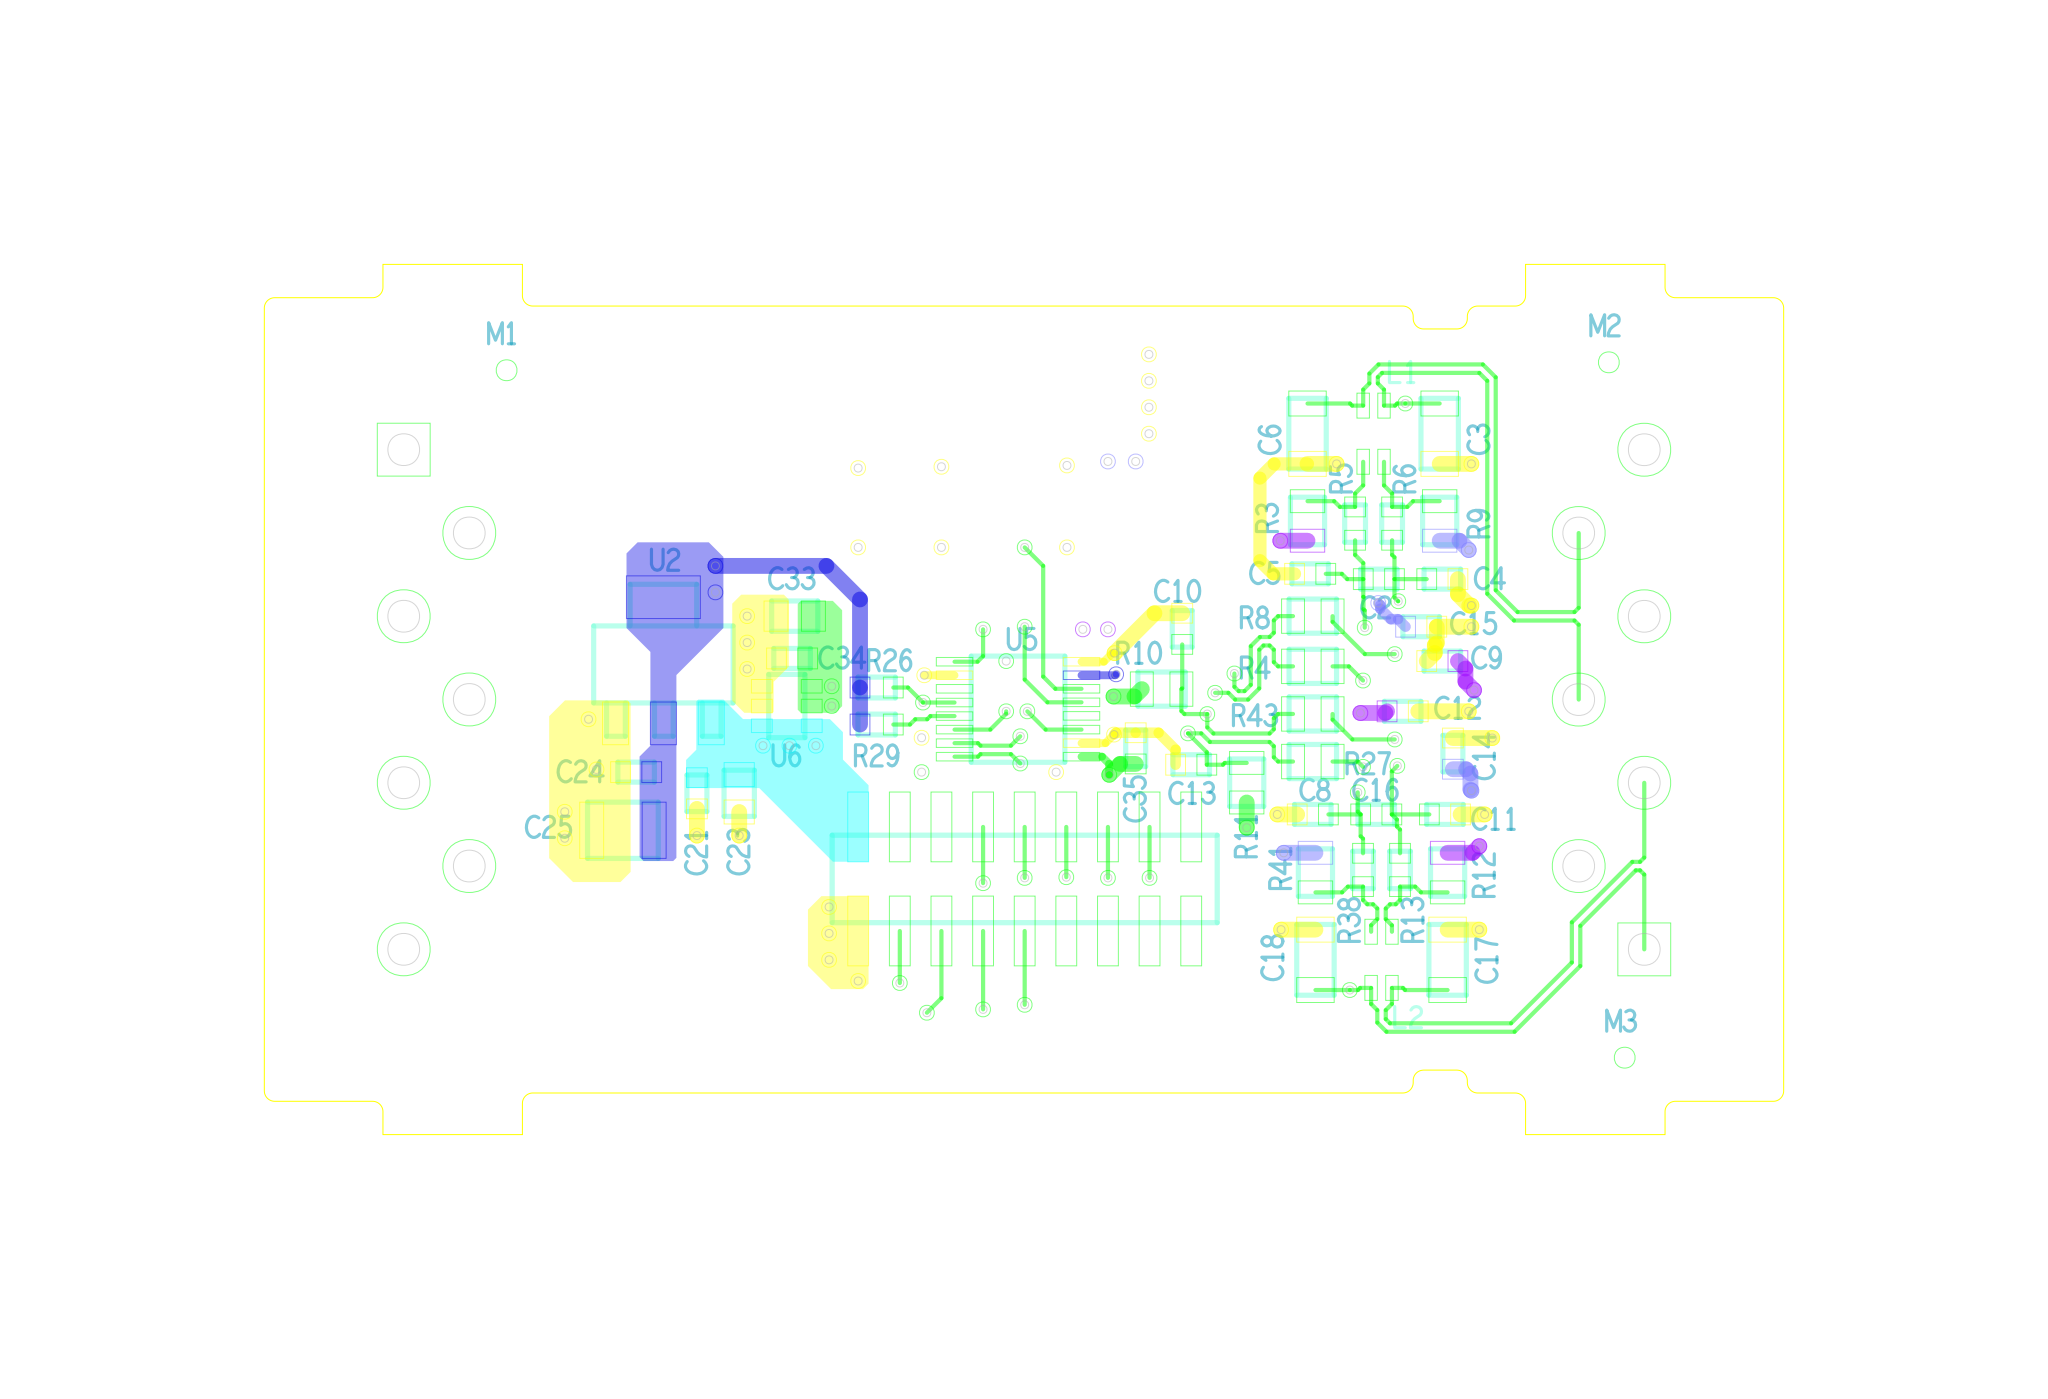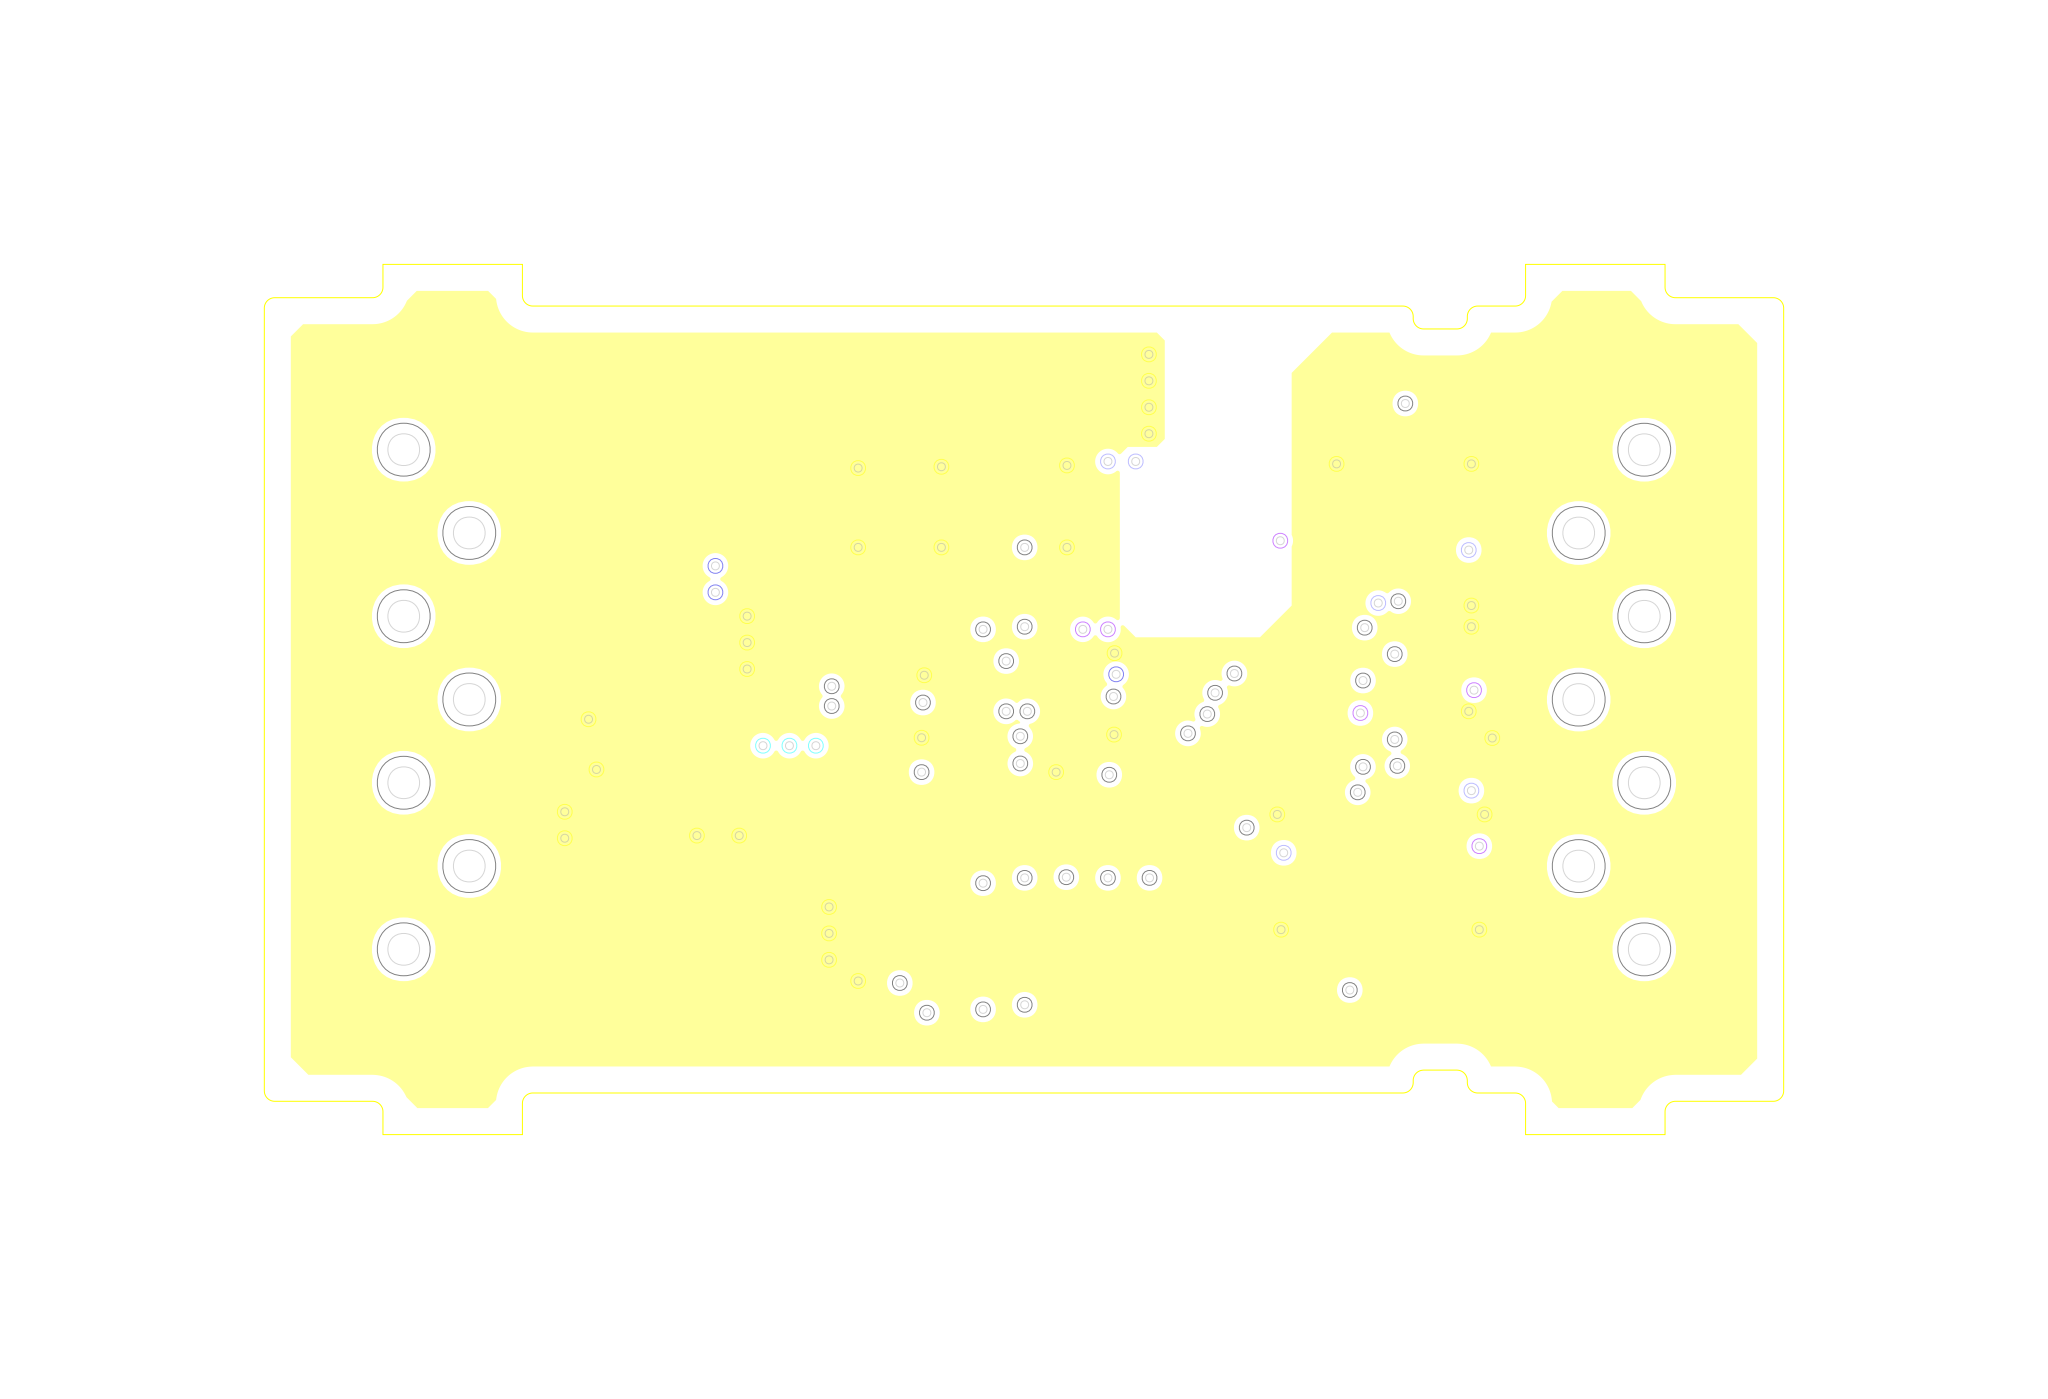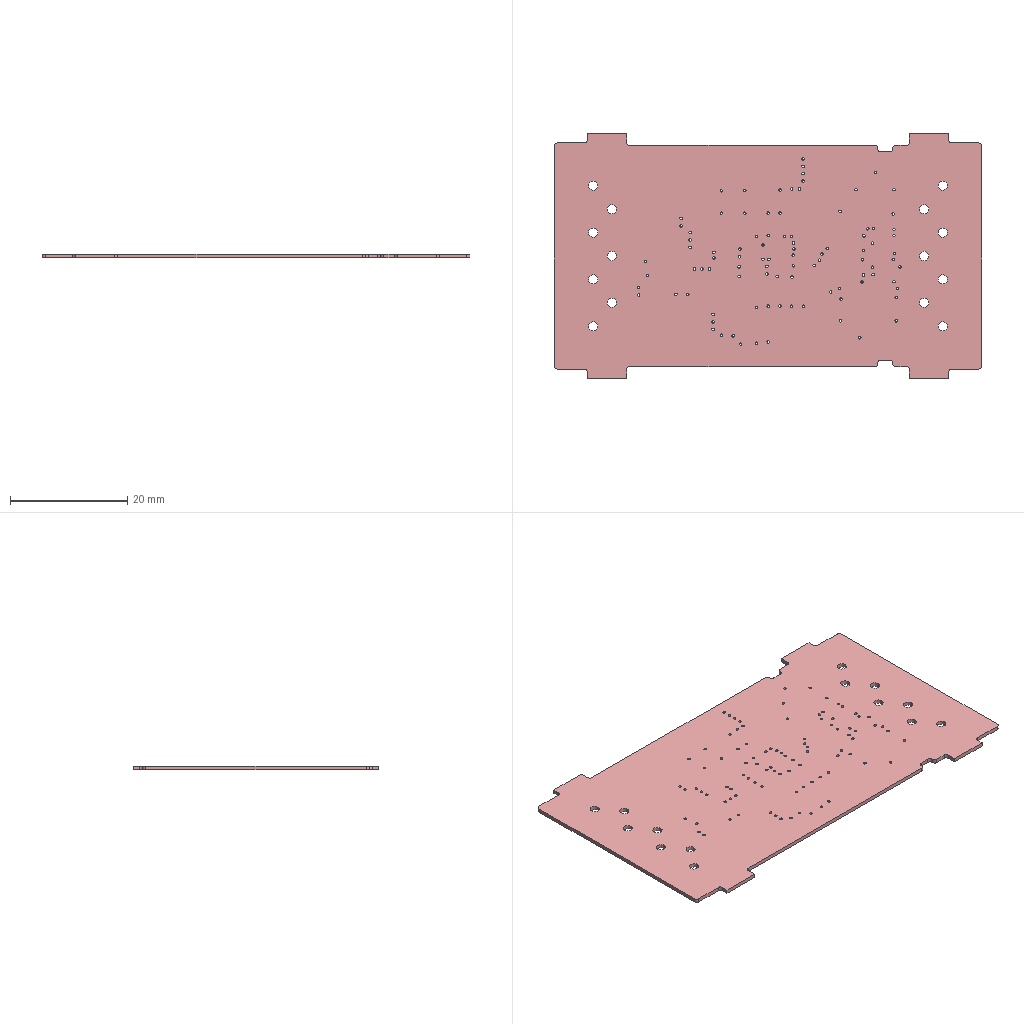Circuit board layout | Cadence Allegro | box 73 x 41.8 x 0.7 mm
Layer stack:
# Cadence Allegro layer stack of  (unit mm; from the constraint file cross-section; dielectric type: 0 not recorded (Allegro does not mark core vs prepreg), 3 surface material)
index,name,kind,layer,copper_thickness_mm,dielectric_type,dielectric_thickness_mm,dielectric_material,dielectric_constant
0,Top Surface,other,,,,,,
1,TOP,copper,TOP,0.0305,,,,
2,Dielectric1,dielectric,,,0,0.2032,FR-4,4.5
3,L2_GND,copper,L2_GND,0.0305,,,,
4,Dielectric2,dielectric,,,0,0.2032,FR-4,4.5
5,L3_PWR,copper,L3_PWR,0.0305,,,,
6,Dielectric3,dielectric,,,0,0.2032,FR-4,4.5
7,BOTTOM,copper,BOTTOM,0.0305,,,,
8,Bottom Surface,other,,,,,,
# drill layer pairs: low layer,high layer
drill_pair,TOP,BOTTOM
Part placement:
REFDES,COMP_VALUE,SYM_NAME,SYM_X,SYM_Y,SYM_ROTATE,SYM_MIRROR
C1,10nF/50V,C0603,4640.0,4190.0,0.000,YES
C2,10nF/50V,C0603,5430.0,4500.0,0.000,NO
C3,1nF/2kV,C1206,5545.0,4775.0,270.000,NO
C4,10nF/50V,C0603,5550.0,4500.0,0.000,NO
C5,10nF/50V,C0603,5300.0,4510.0,180.000,NO
C6,1nF/2kV,C1206,5295.0,4775.0,270.000,NO
C7,10nF/50V,C0603,4790.0,4090.0,180.000,YES
C8,10nF/50V,C0603,5305.0,4055.0,180.000,NO
C9,100nF/50V,C0603,5550.0,4345.0,180.000,NO
C10,10nF/50V,C0603,5058.0,4406.0,90.000,NO
C11,10nF/50V,C0603,5555.0,4055.0,0.000,NO
C12,100nF/50V,C0603,5475.0,4250.0,0.000,NO
C13,10nF/50V,C0603,5075.0,4149.0,180.000,NO
C14,100nF/50V,C0603,5570.0,4170.0,90.000,NO
C15,100nF/50V,C0603,5510.0,4410.0,0.000,NO
C16,10nF/50V,C0603,5425.0,4055.0,180.000,NO
C17,1nF/2kV,C1206,5560.0,3780.0,90.000,NO
C18,1nF/2kV,C1206,5310.0,3780.0,90.000,NO
C21,100nF/50V,C0603,4140.0,4095.0,270.000,NO
C22,1nF/2kV,C1206,5100.0,4790.0,180.000,YES
C23,10uF/25V,C0805,4220.0,4095.0,270.000,NO
C24,100nF/50V,C0603,4025.0,4135.0,180.000,NO
C25,22uF/16V,C1210,4000.0,4025.0,180.000,NO
C33,10uF/25V,C0805,4325.0,4430.0,180.000,NO
C34,100nF/50V,C0603,4320.0,4350.0,180.000,NO
C35,1uF/16V,C0603,4970.0,4180.0,90.000,NO
C36,100nF/50V,C0603,4315.0,4345.0,0.000,YES
C37,100nF/50V,C0603,4975.0,4335.0,270.000,YES
C38,10uF/25V,C0805,5055.0,4335.0,270.000,YES
C41,1uF/16V,C0603,4315.0,4270.0,0.000,YES
D1,SI2318CDS,SOT23,5525.0,4775.5,0.000,YES
D2,SI2318CDS,SOT23,5315.0,3769.5,180.000,YES
J1,0162-A107,CON7-0162-A107,5932.0,3799.8,90.000,NO
J2,TW-09-04-T-D-300-SM,CON18-TW-09,4760.0,3933.0,0.000,NO
J3,0162-A107,CON7-0162-A107,3585.4,4744.8,270.000,NO
J5,SQW-111-01-F-D-VS,CON22-SQW-111,4760.0,4560.0,180.000,YES
L1,260R-744232261,744232261,5420.0,4775.0,270.000,NO
L2,260R-744232261,744232261,5435.0,3780.0,90.000,NO
M1,MARK-BOARD,MARKPOINT-BOARD,3780.0,4895.0,0.000,NO
M2,MARK-BOARD,MARKPOINT-BOARD,5865.0,4910.0,0.000,NO
M3,MARK-BOARD,MARKPOINT-BOARD,5895.0,3595.0,0.000,NO
M4,MARK-BOARD,MARKPOINT-BOARD,3780.0,4895.0,0.000,YES
M5,MARK-BOARD,MARKPOINT-BOARD,5865.0,4910.0,0.000,YES
M6,MARK-BOARD,MARKPOINT-BOARD,5895.0,3595.0,0.000,YES
R1,2.6K-0.1%,R0805,4665.0,4295.0,90.000,YES
R2,2.6K-0.1%,R0805,4645.0,4105.0,180.000,YES
R3,10M-1/8W,R0805,5295.0,4610.0,90.000,NO
R4,19.5K-0.1%,R0805,5305.0,4335.0,180.000,NO
R5,15K-1/10W,R0603,5385.0,4605.0,270.000,NO
R6,15K-1/10W,R0603,5455.0,4605.0,270.000,NO
R7,250-0.1%,R0805,5425.0,4630.0,270.000,YES
R8,19.5K-0.1%,R0805,5305.0,4430.0,180.000,NO
R9,10M-1/8W,R0805,5545.0,4610.0,270.000,NO
R10,2.6K-0.1%,R0805,5019.0,4292.0,0.000,NO
R11,2.6K-0.1%,R0805,5180.0,4115.0,90.000,NO
R12,10M-1/8W,R0805,5560.0,3945.0,270.000,NO
R13,15K-1/10W,R0603,5470.0,3950.0,90.000,NO
R17,1M-1/4W,R1210,5100.0,4910.0,180.000,YES
R26,10K-1/10W,R0603,4480.0,4295.0,0.000,NO
R27,19.5K-0.1%,R0805,5305.0,4155.0,180.000,NO
R28,250-0.1%,R0805,5430.0,3925.0,90.000,YES
R29,10K-1/10W,R0603,4480.0,4225.0,0.000,NO
R38,15K-1/10W,R0603,5400.0,3950.0,90.000,NO
R41,10M-1/8W,R0805,5310.0,3945.0,90.000,NO
R43,19.5K-0.1%,R0805,5305.0,4245.0,180.000,NO
R44,0-1/10W,R0603,5425.0,4785.0,270.000,YES
R45,0-1/10W,R0603,5430.0,3770.0,90.000,YES
U1,LM358MX/NOPB,SO8,5427.6,4383.4,180.000,YES
U2,U-LM1117IMPX-3.3/NOPB,SOT223,4076.6,4346.5,0.000,NO
U5,AD7705BRU,TSSOP16_P0_65,4747.4,4254.0,0.000,NO
U6,REF3425IDBVR,SOT23_6,4310.0,4260.0,0.000,NO
U7,LM358MX/NOPB,SO8,5427.4,4171.6,0.000,YES
Pad and via stacks:
# Allegro (Cadence) via spans and padstacks; design units: ("mils" 1 10)
# via spans: padstack,start_layer,end_layer,net_example,count
VIA,ETCH/TOP,ETCH/BOTTOM,GND,94
# Allegro padstack definitions: name,start_layer,end_layer,drill,plating,holeType,type
SMD0_95X1_00,"ETCH/TOP","ETCH/TOP",0.0,"PLATED","none","smd"
SMD1_20X1_80,"ETCH/TOP","ETCH/TOP",0.0,"PLATED","none","smd"
SMD1_15X1_45,"ETCH/TOP","ETCH/TOP",0.0,"PLATED","none","smd"
SMD1_15X2_70,"ETCH/TOP","ETCH/TOP",0.0,"PLATED","none","smd"
SMD20_17,"ETCH/TOP","ETCH/TOP",0.0,"PLATED","none","smd"
SMDREC_132X40,"ETCH/TOP","ETCH/TOP",0.0,"PLATED","none","smd"
SMDREC_96X40,"ETCH/TOP","ETCH/TOP",0.0,"NON_PLATED","none","smd"
SMD0_60X1_20,"ETCH/TOP","ETCH/TOP",0.0,"PLATED","none","smd"
SOLDERMASK_40_80,"ETCH/TOP","ETCH/TOP",0.0,"NON_PLATED","none","smd"
SMD1_10X1_65,"ETCH/TOP","ETCH/TOP",0.0,"PLATED","none","smd"
SMD1_10X2_80,"ETCH/TOP","ETCH/TOP",0.0,"PLATED","none","smd"
SMD2_25X0_66,"ETCH/TOP","ETCH/TOP",0.0,"PLATED","none","smd"
SMD1_25X2_05,"ETCH/TOP","ETCH/TOP",0.0,"PLATED","none","smd"
SMD3_55X2_05,"ETCH/TOP","ETCH/TOP",0.0,"PLATED","none","smd"
SMD1_75X0_41,"ETCH/TOP","ETCH/TOP",0.0,"PLATED","none","smd"
SMD1_00X0_65,"ETCH/TOP","ETCH/TOP",0.0,"PLATED","none","smd"
THRSQR_60X100,"ETCH/TOP","ETCH/BOTTOM",60.0,"PLATED","circle_drill","through"
THRCIR_60X100,"ETCH/TOP","ETCH/BOTTOM",60.0,"PLATED","circle_drill","through"
VIA,"ETCH/TOP","ETCH/BOTTOM",15.0,"PLATED","circle_drill","through"
Design rules, without the lines most boards share, first 16 of 33 lines:
# Cadence Allegro design rules of  (from the Constraint Manager export constraints.dcfx, design unit mil; typed fields in mm)
# columns: name | kind | enabled | priority | scope1 | scope2 | descriptor | typed fields (field=value)
# Allegro precedence (priority 1 wins): 1 Region class-to-class, 2 Region class, 3 Region, 4 class-to-class, 5 DiffPair/Bus/NetGroup override, 6 NetClass, 7 constraint set (CSet) default
# per-layer values are written LAYER=value in the descriptor and LAYER:mm in the typed field; a maximum of 0 means no limit set
# --- net classes (and buses / net groups) ---
# (no net classes defined: every net uses the default constraint sets)
# --- track widths, neck and differential-pair gap (physical constraint sets) ---
DEFAULT | PhysicalCSet | enabled | 7 | Design default | All | Physical Constraint (Min Line Width=8mil) (Max Line Width=0mil) (Min Neck Width=8mil) (Max Neck Length=0mil) (DiffPair Primary Gap=8mil) (DiffPair Neck Gap=0mil) (DiffPair Min Space=8mil) (DiffPair Coupled +Tol=0mil) (DiffPair Coupled -Tol=0mil) (Min BB Via Stagger=5mil) (Max BB Via Stagger=0mil) (T-junctions=ANYWHERE) (Pad-pad direct connect=ALL_ALLOWED) (Allowed vias=VIA) | min_line_width=0.2032 min_neck_width=0.2032 min_bvia_stagger=0.127 max_bvia_stagger=0 ts_allowed=ANYWHERE diffp_primary_gap=0.2032 diffp_neck_gap=0 max_line_width=0 maximum_neck_length=0 pad_pad_direct_connect=ALL_ALLOWED allow_on_etch_subclass=TRUE diffp_coupled_plus=0 diffp_coupled_minus=0 diffp_min_space=0.2032 vias=VIA
# --- clearances: line / pad / via / shape / hole (spacing constraint sets) ---
DEFAULT | SpacingCSet | enabled | 7 | Design default | All | Clearance Constraint (Line-Line=10mil) (Line-SMD Pad=10mil) (Line-Thru Pin=10mil) (Line-Via=10mil) (Line-Shape=TOP=10mil L2_GND=10mil L3_PWR=25mil BOTTOM=10mil) (SMD Pad-SMD Pad=9mil) (Thru Pin-Thru Pin=10mil) (Thru Pin-SMD Pad=10mil) (SMD Pad-Via=10mil) (Thru Pin-Via=10mil) (Via-Via=10mil) (Shape-SMD Pad=10mil) (Shape-Thru Pin=10mil) (Shape-Via=10mil) (Shape-Shape=10mil) (Hole-Hole=10mil) (Hole-Line=10mil) (Hole-Shape=10mil) (BB Via-BB Via=10mil) (uVia-uVia=10mil) | thrupin_to_thrupin_spacing=0.254 thrupin_to_smdpin_spacing=0.254 thrupin_to_thruvia_spacing=0.254 line_to_thrupin_spacing=0.254 thrupin_to_shape_spacing=0.254 smdpin_to_smdpin_spacing=0.2286 smdpin_to_thruvia_spacing=0.254 line_to_smdpin_spacing=0.254 shape_to_smdpin_spacing=0.254 thruvia_to_thruvia_spacing=0.254 line_to_thruvia_spacing=0.254 shape_to_thruvia_spacing=0.254 line_to_line_spacing=0.254 line_to_shape_spacing=TOP:0.254,L2_GND:0.254,L3_PWR:0.635,BOTTOM:0.254 shape_to_shape_spacing=0.254 bbv_to_bbv_spacing=0.254 bbv_to_thrupin_spacing=0.254 bbv_to_smdpin_spacing=0.254 bbv_to_thruvia_spacing=0.254 bbv_to_line_spacing=0.254 bbv_to_shape_spacing=0.254 bbv_to_testpin_spacing=0.254 bbv_to_testvia_spacing=0.254 testpin_to_testpin_spacing=0.254 testpin_to_thrupin_spacing=0.254 smdpin_to_testpin_spacing=0.254 testpin_to_thruvia_spacing=0.254 testpin_to_testvia_spacing=0.254 line_to_testpin_spacing=0.254 shape_to_testpin_spacing=0.254 testvia_to_testvia_spacing=0.254 testvia_to_thrupin_spacing=0.254 smdpin_to_testvia_spacing=0.254 testvia_to_thruvia_spacing=0.254 line_to_testvia_spacing=0.254 shape_to_testvia_spacing=0.254 bondpad_to_bondpad_spacing=0.254 thrupin_to_bondpad_spacing=0.254 smdpin_to_bondpad_spacing=0.254 bondpad_to_thruvia_spacing=0.254 bondpad_to_line_spacing=0.254 bondpad_to_shape_spacing=0.254 bondpad_to_bbv_spacing=0.254 bondpad_to_testpin_spacing=0.254 bondpad_to_testvia_spacing=0.254 min_bvia_gap=0.254 hole_to_pin_spacing=0.254 hole_to_via_spacing=0.254 hole_to_line_spacing=0.254 hole_to_shape_spacing=0.254 hole_to_hole_spacing=0.254 mvia_to_mvia_spacing=0.254 mvia_to_thrupin_spacing=0.254 mvia_to_smdpin_spacing=0.254 mvia_to_thruvia_spacing=0.254 mvia_to_bbv_spacing=0.254 mvia_to_line_spacing=0.254 mvia_to_shape_spacing=0.254 mvia_to_testpin_spacing=0.254 mvia_to_testvia_spacing=0.254 bondpad_to_mvia_spacing=0.254 bondpad_to_bondpad_diffp_spc=0.127
DEFAULT | SameNetSpacingCSet | enabled | 7 | Design default | All | Same-Net Clearance (Line-Line=5mil) (Line-SMD Pad=5mil) (Line-Thru Pin=5mil) (Line-Via=5mil) (Line-Shape=5mil) (SMD Pad-SMD Pad=5mil) (Thru Pin-Thru Pin=5mil) (Thru Pin-SMD Pad=5mil) (SMD Pad-Via=5mil) (Thru Pin-Via=5mil) (Via-Via=5mil) (Shape-SMD Pad=5mil) (Shape-Thru Pin=5mil) (Shape-Via=5mil) (Shape-Shape=5mil) (Hole-Hole=8mil) (Hole-Line=8mil) (Hole-Shape=8mil) (BB Via-BB Via=5mil) (uVia-uVia=5mil) | sn_thrupin_to_thrupin_spacing=0.127 sn_thrupin_to_smdpin_spacing=0.127 sn_thrupin_to_thruvia_spacing=0.127 sn_line_to_thrupin_spacing=0.127 sn_thrupin_to_shape_spacing=0.127 sn_smdpin_to_smdpin_spacing=0.127 sn_smdpin_to_thruvia_spacing=0.127 sn_line_to_smdpin_spacing=0.127 sn_shape_to_smdpin_spacing=0.127 sn_thruvia_to_thruvia_spacing=0.127 sn_line_to_thruvia_spacing=0.127 sn_shape_to_thruvia_spacing=0.127 sn_line_to_line_spacing=0.127 sn_line_to_shape_spacing=0.127 sn_shape_to_shape_spacing=0.127 sn_bbv_to_bbv_spacing=0.127 sn_bbv_to_thrupin_spacing=0.127 sn_bbv_to_smdpin_spacing=0.127 sn_bbv_to_thruvia_spacing=0.127 sn_bbv_to_line_spacing=0.127 sn_bbv_to_shape_spacing=0.127 sn_bbv_to_testpin_spacing=0.127 sn_bbv_to_testvia_spacing=0.127 sn_testpin_to_testpin_spacing=0.127 sn_testpin_to_thrupin_spacing=0.127 sn_smdpin_to_testpin_spacing=0.127 sn_testpin_to_thruvia_spacing=0.127 sn_testpin_to_testvia_spacing=0.127 sn_line_to_testpin_spacing=0.127 sn_shape_to_testpin_spacing=0.127 sn_testvia_to_testvia_spacing=0.127 sn_testvia_to_thrupin_spacing=0.127 sn_smdpin_to_testvia_spacing=0.127 sn_testvia_to_thruvia_spacing=0.127 sn_line_to_testvia_spacing=0.127 sn_shape_to_testvia_spacing=0.127 sn_bondpad_to_bondpad_spacing=0.127 sn_thrupin_to_bondpad_spacing=0.127 sn_smdpin_to_bondpad_spacing=0.127 sn_bondpad_to_thruvia_spacing=0.127 sn_bondpad_to_line_spacing=0.127 sn_bondpad_to_shape_spacing=0.127 sn_bondpad_to_bbv_spacing=0.127 sn_bondpad_to_testpin_spacing=0.127 sn_bondpad_to_testvia_spacing=0.127 same_net=TRUE sn_hole_to_pin_spacing=0.2032 sn_hole_to_via_spacing=0.2032 sn_hole_to_line_spacing=0.2032 sn_hole_to_shape_spacing=0.2032 sn_hole_to_hole_spacing=0.2032 sn_mvia_to_mvia_spacing=0.127 sn_mvia_to_thrupin_spacing=0.127 sn_mvia_to_smdpin_spacing=0.127 sn_mvia_to_thruvia_spacing=0.127 sn_mvia_to_bbv_spacing=0.127 sn_mvia_to_line_spacing=0.127 sn_mvia_to_shape_spacing=0.127 sn_mvia_to_testpin_spacing=0.127 sn_mvia_to_testvia_spacing=0.127 sn_bondpad_to_mvia_spacing=0.127
# --- differential pairs (10) ---
DIFFPAIR7 | DiffPair | enabled | 5 | N7791248 | N7791211 | Differential Pair (Primary Gap=8mil) (Min Line Width=8mil) (Physical CSet=DEFAULT) | gap=0.2032 width=0.2032
DIFFPAIR6 | DiffPair | enabled | 5 | N7790913 | N7790885 | Differential Pair (Primary Gap=8mil) (Min Line Width=8mil) (Physical CSet=DEFAULT) | gap=0.2032 width=0.2032
DIFFPAIR5 | DiffPair | enabled | 5 | N7791207 | N7791236 | Differential Pair (Primary Gap=8mil) (Min Line Width=8mil) (Physical CSet=DEFAULT) | gap=0.2032 width=0.2032
DIFFPAIR4 | DiffPair | enabled | 5 | N7794115 | N7794091 | Differential Pair (Primary Gap=8mil) (Min Line Width=8mil) (Physical CSet=DEFAULT) | gap=0.2032 width=0.2032